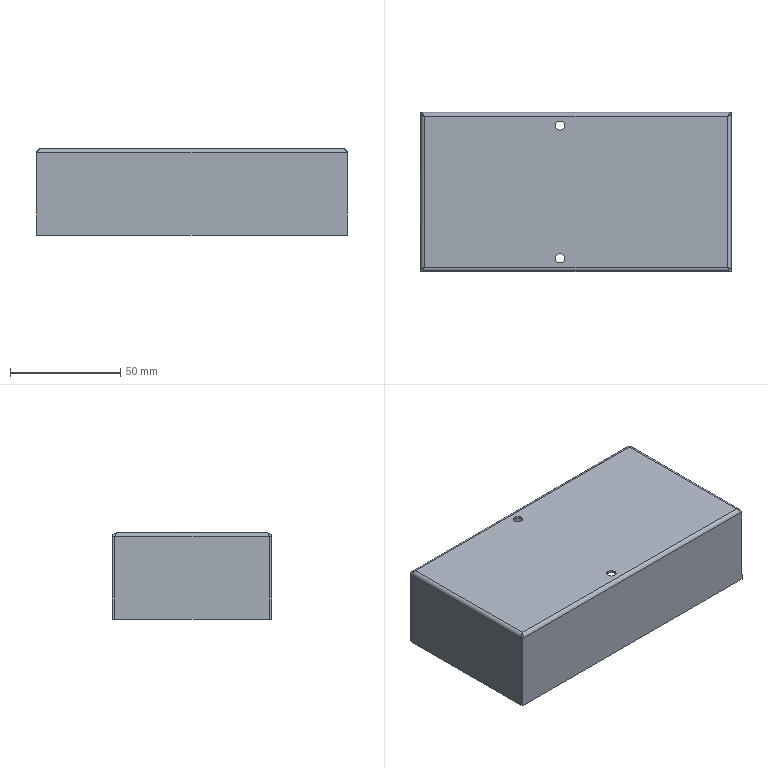Part | STEP file | 复件 FHB175-018^FHB175S-PRW-P40(马达RightUpper折-400W伺服电机) | 1 solid | 42 faces | box 140.5 x 72 x 39 mm | volume 25843 mm3 | plane 22 | cylinder 12 | spline 8 | commonest cylinder face diameters 1.473 x4 3.473 x4 4.2 x4